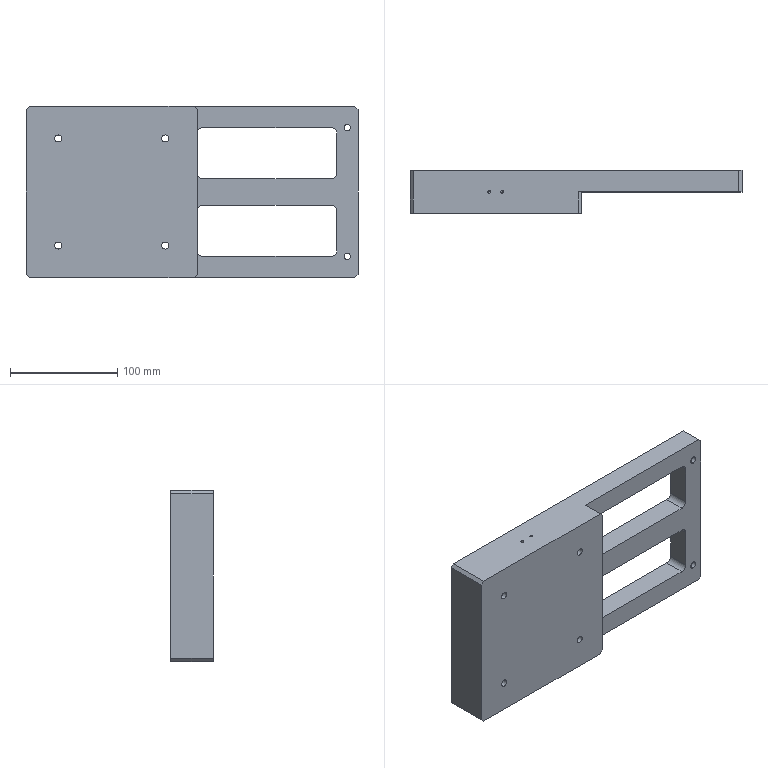Part | 1 solid | 56 faces | box 310 x 40 x 160 mm | volume 1242142 mm3 | plane 24 | cylinder 24 | cone 8 | commonest cylinder face diameters 10 x8 6.6 x4 6.8 x4 11 x4 2.5 x2 6 x2
STEP:
#1=CARTESIAN_POINT('',(125.,20.,60.));
#2=VERTEX_POINT('',#1);
#3=CARTESIAN_POINT('',(5.,20.,60.));
#4=VERTEX_POINT('',#3);
#5=CARTESIAN_POINT('',(5.,20.,60.));
#6=DIRECTION('',(-1.,0.,0.));
#7=VECTOR('',#6,1000.);
#8=LINE('',#5,#7);
#9=EDGE_CURVE('',#2,#4,#8,.T.);
#10=ORIENTED_EDGE('',*,*,#9,.T.);
#11=CARTESIAN_POINT('',(5.,40.,60.));
#12=VERTEX_POINT('',#11);
#13=CARTESIAN_POINT('',(5.,40.,60.));
#14=DIRECTION('',(0.,-1.,0.));
#15=VECTOR('',#14,1000.);
#16=LINE('',#13,#15);
#17=EDGE_CURVE('',#12,#4,#16,.T.);
#18=ORIENTED_EDGE('',*,*,#17,.F.);
#19=CARTESIAN_POINT('',(125.,40.,60.));
#20=VERTEX_POINT('',#19);
#21=CARTESIAN_POINT('',(5.,40.,60.));
#22=DIRECTION('',(-1.,0.,0.));
#23=VECTOR('',#22,1000.);
#24=LINE('',#21,#23);
#25=EDGE_CURVE('',#20,#12,#24,.T.);
#26=ORIENTED_EDGE('',*,*,#25,.F.);
#27=CARTESIAN_POINT('',(125.,40.,60.));
#28=DIRECTION('',(0.,-1.,0.));
#29=VECTOR('',#28,1000.);
#30=LINE('',#27,#29);
#31=EDGE_CURVE('',#20,#2,#30,.T.);
#32=ORIENTED_EDGE('',*,*,#31,.T.);
#33=EDGE_LOOP('',(#10,#18,#26,#32));
#34=FACE_BOUND('',#33,.T.);
#35=CARTESIAN_POINT('',(5.,40.,60.));
#36=DIRECTION('',(0.,0.,1.));
#37=DIRECTION('',(1.,0.,0.));
#38=AXIS2_PLACEMENT_3D('',#35,#36,#37);
#39=PLANE('',#38);
#40=ADVANCED_FACE('',(#34),#39,.F.);
#41=CARTESIAN_POINT('',(0.,20.,55.));
#42=VERTEX_POINT('',#41);
#43=CARTESIAN_POINT('',(5.,20.,55.));
#44=DIRECTION('',(0.,-1.,0.));
#45=DIRECTION('',(0.,0.,1.));
#46=AXIS2_PLACEMENT_3D('',#43,#44,#45);
#47=CIRCLE('',#46,5.);
#48=EDGE_CURVE('',#4,#42,#47,.T.);
#49=ORIENTED_EDGE('',*,*,#48,.T.);
#50=CARTESIAN_POINT('',(0.,40.,55.));
#51=VERTEX_POINT('',#50);
#52=CARTESIAN_POINT('',(0.,40.,55.));
#53=DIRECTION('',(0.,-1.,0.));
#54=VECTOR('',#53,1000.);
#55=LINE('',#52,#54);
#56=EDGE_CURVE('',#51,#42,#55,.T.);
#57=ORIENTED_EDGE('',*,*,#56,.F.);
#58=CARTESIAN_POINT('',(5.,40.,55.));
#59=DIRECTION('',(0.,-1.,0.));
#60=DIRECTION('',(0.,0.,1.));
#61=AXIS2_PLACEMENT_3D('',#58,#59,#60);
#62=CIRCLE('',#61,5.);
#63=EDGE_CURVE('',#12,#51,#62,.T.);
#64=ORIENTED_EDGE('',*,*,#63,.F.);
#65=ORIENTED_EDGE('',*,*,#17,.T.);
#66=EDGE_LOOP('',(#49,#57,#64,#65));
#67=FACE_BOUND('',#66,.T.);
#68=CARTESIAN_POINT('',(5.,40.,55.));
#69=DIRECTION('',(0.,-1.,0.));
#70=DIRECTION('',(0.,0.,-1.));
#71=AXIS2_PLACEMENT_3D('',#68,#69,#70);
#72=CYLINDRICAL_SURFACE('',#71,5.);
#73=ADVANCED_FACE('',(#67),#72,.F.);
#74=CARTESIAN_POINT('',(0.,20.,17.5));
#75=VERTEX_POINT('',#74);
#76=CARTESIAN_POINT('',(5.,20.,12.5));
#77=VERTEX_POINT('',#76);
#78=CARTESIAN_POINT('',(5.,20.,17.5));
#79=DIRECTION('',(0.,-1.,0.));
#80=DIRECTION('',(0.,0.,1.));
#81=AXIS2_PLACEMENT_3D('',#78,#79,#80);
#82=CIRCLE('',#81,5.);
#83=EDGE_CURVE('',#75,#77,#82,.T.);
#84=ORIENTED_EDGE('',*,*,#83,.T.);
#85=CARTESIAN_POINT('',(5.,40.,12.5));
#86=VERTEX_POINT('',#85);
#87=CARTESIAN_POINT('',(5.,40.,12.5));
#88=DIRECTION('',(0.,-1.,0.));
#89=VECTOR('',#88,1000.);
#90=LINE('',#87,#89);
#91=EDGE_CURVE('',#86,#77,#90,.T.);
#92=ORIENTED_EDGE('',*,*,#91,.F.);
#93=CARTESIAN_POINT('',(0.,40.,17.5));
#94=VERTEX_POINT('',#93);
#95=CARTESIAN_POINT('',(5.,40.,17.5));
#96=DIRECTION('',(0.,-1.,0.));
#97=DIRECTION('',(0.,0.,1.));
#98=AXIS2_PLACEMENT_3D('',#95,#96,#97);
#99=CIRCLE('',#98,5.);
#100=EDGE_CURVE('',#94,#86,#99,.T.);
#101=ORIENTED_EDGE('',*,*,#100,.F.);
#102=CARTESIAN_POINT('',(0.,40.,17.5));
#103=DIRECTION('',(0.,-1.,0.));
#104=VECTOR('',#103,1000.);
#105=LINE('',#102,#104);
#106=EDGE_CURVE('',#94,#75,#105,.T.);
#107=ORIENTED_EDGE('',*,*,#106,.T.);
#108=EDGE_LOOP('',(#84,#92,#101,#107));
#109=FACE_BOUND('',#108,.T.);
#110=CARTESIAN_POINT('',(5.,40.,17.5));
#111=DIRECTION('',(0.,-1.,0.));
#112=DIRECTION('',(0.,0.,-1.));
#113=AXIS2_PLACEMENT_3D('',#110,#111,#112);
#114=CYLINDRICAL_SURFACE('',#113,5.);
#115=ADVANCED_FACE('',(#109),#114,.F.);
#116=CARTESIAN_POINT('',(125.,20.,12.5));
#117=VERTEX_POINT('',#116);
#118=CARTESIAN_POINT('',(5.,20.,12.5));
#119=DIRECTION('',(1.,0.,0.));
#120=VECTOR('',#119,1000.);
#121=LINE('',#118,#120);
#122=EDGE_CURVE('',#77,#117,#121,.T.);
#123=ORIENTED_EDGE('',*,*,#122,.T.);
#124=CARTESIAN_POINT('',(125.,40.,12.5));
#125=VERTEX_POINT('',#124);
#126=CARTESIAN_POINT('',(125.,40.,12.5));
#127=DIRECTION('',(0.,-1.,0.));
#128=VECTOR('',#127,1000.);
#129=LINE('',#126,#128);
#130=EDGE_CURVE('',#125,#117,#129,.T.);
#131=ORIENTED_EDGE('',*,*,#130,.F.);
#132=CARTESIAN_POINT('',(5.,40.,12.5));
#133=DIRECTION('',(1.,0.,0.));
#134=VECTOR('',#133,1000.);
#135=LINE('',#132,#134);
#136=EDGE_CURVE('',#86,#125,#135,.T.);
#137=ORIENTED_EDGE('',*,*,#136,.F.);
#138=ORIENTED_EDGE('',*,*,#91,.T.);
#139=EDGE_LOOP('',(#123,#131,#137,#138));
#140=FACE_BOUND('',#139,.T.);
#141=CARTESIAN_POINT('',(5.,40.,12.5));
#142=DIRECTION('',(0.,0.,-1.));
#143=DIRECTION('',(-1.,0.,0.));
#144=AXIS2_PLACEMENT_3D('',#141,#142,#143);
#145=PLANE('',#144);
#146=ADVANCED_FACE('',(#140),#145,.F.);
#147=CARTESIAN_POINT('',(130.,20.,17.5));
#148=VERTEX_POINT('',#147);
#149=CARTESIAN_POINT('',(125.,20.,17.5));
#150=DIRECTION('',(0.,-1.,0.));
#151=DIRECTION('',(0.,0.,-1.));
#152=AXIS2_PLACEMENT_3D('',#149,#150,#151);
#153=CIRCLE('',#152,5.);
#154=EDGE_CURVE('',#117,#148,#153,.T.);
#155=ORIENTED_EDGE('',*,*,#154,.T.);
#156=CARTESIAN_POINT('',(130.,40.,17.5));
#157=VERTEX_POINT('',#156);
#158=CARTESIAN_POINT('',(130.,40.,17.5));
#159=DIRECTION('',(0.,-1.,0.));
#160=VECTOR('',#159,1000.);
#161=LINE('',#158,#160);
#162=EDGE_CURVE('',#157,#148,#161,.T.);
#163=ORIENTED_EDGE('',*,*,#162,.F.);
#164=CARTESIAN_POINT('',(125.,40.,17.5));
#165=DIRECTION('',(0.,-1.,0.));
#166=DIRECTION('',(0.,0.,-1.));
#167=AXIS2_PLACEMENT_3D('',#164,#165,#166);
#168=CIRCLE('',#167,5.);
#169=EDGE_CURVE('',#125,#157,#168,.T.);
#170=ORIENTED_EDGE('',*,*,#169,.F.);
#171=ORIENTED_EDGE('',*,*,#130,.T.);
#172=EDGE_LOOP('',(#155,#163,#170,#171));
#173=FACE_BOUND('',#172,.T.);
#174=CARTESIAN_POINT('',(125.,40.,17.5));
#175=DIRECTION('',(0.,-1.,0.));
#176=DIRECTION('',(0.,0.,-1.));
#177=AXIS2_PLACEMENT_3D('',#174,#175,#176);
#178=CYLINDRICAL_SURFACE('',#177,5.);
#179=ADVANCED_FACE('',(#173),#178,.F.);
#180=CARTESIAN_POINT('',(130.,20.,55.));
#181=VERTEX_POINT('',#180);
#182=CARTESIAN_POINT('',(130.,20.,17.5));
#183=DIRECTION('',(0.,0.,1.));
#184=VECTOR('',#183,1000.);
#185=LINE('',#182,#184);
#186=EDGE_CURVE('',#148,#181,#185,.T.);
#187=ORIENTED_EDGE('',*,*,#186,.T.);
#188=CARTESIAN_POINT('',(130.,40.,55.));
#189=VERTEX_POINT('',#188);
#190=CARTESIAN_POINT('',(130.,40.,55.));
#191=DIRECTION('',(0.,-1.,0.));
#192=VECTOR('',#191,1000.);
#193=LINE('',#190,#192);
#194=EDGE_CURVE('',#189,#181,#193,.T.);
#195=ORIENTED_EDGE('',*,*,#194,.F.);
#196=CARTESIAN_POINT('',(130.,40.,17.5));
#197=DIRECTION('',(0.,0.,1.));
#198=VECTOR('',#197,1000.);
#199=LINE('',#196,#198);
#200=EDGE_CURVE('',#157,#189,#199,.T.);
#201=ORIENTED_EDGE('',*,*,#200,.F.);
#202=ORIENTED_EDGE('',*,*,#162,.T.);
#203=EDGE_LOOP('',(#187,#195,#201,#202));
#204=FACE_BOUND('',#203,.T.);
#205=CARTESIAN_POINT('',(130.,40.,17.5));
#206=DIRECTION('',(1.,0.,0.));
#207=DIRECTION('',(0.,0.,-1.));
#208=AXIS2_PLACEMENT_3D('',#205,#206,#207);
#209=PLANE('',#208);
#210=ADVANCED_FACE('',(#204),#209,.F.);
#211=CARTESIAN_POINT('',(125.,20.,55.));
#212=DIRECTION('',(0.,-1.,0.));
#213=DIRECTION('',(0.,0.,1.));
#214=AXIS2_PLACEMENT_3D('',#211,#212,#213);
#215=CIRCLE('',#214,5.);
#216=EDGE_CURVE('',#181,#2,#215,.T.);
#217=ORIENTED_EDGE('',*,*,#216,.T.);
#218=ORIENTED_EDGE('',*,*,#31,.F.);
#219=CARTESIAN_POINT('',(125.,40.,55.));
#220=DIRECTION('',(0.,-1.,0.));
#221=DIRECTION('',(0.,0.,1.));
#222=AXIS2_PLACEMENT_3D('',#219,#220,#221);
#223=CIRCLE('',#222,5.);
#224=EDGE_CURVE('',#189,#20,#223,.T.);
#225=ORIENTED_EDGE('',*,*,#224,.F.);
#226=ORIENTED_EDGE('',*,*,#194,.T.);
#227=EDGE_LOOP('',(#217,#218,#225,#226));
#228=FACE_BOUND('',#227,.T.);
#229=CARTESIAN_POINT('',(125.,40.,55.));
#230=DIRECTION('',(0.,-1.,0.));
#231=DIRECTION('',(0.,0.,-1.));
#232=AXIS2_PLACEMENT_3D('',#229,#230,#231);
#233=CYLINDRICAL_SURFACE('',#232,5.);
#234=ADVANCED_FACE('',(#228),#233,.F.);
#235=CARTESIAN_POINT('',(5.,20.,-60.));
#236=VERTEX_POINT('',#235);
#237=CARTESIAN_POINT('',(125.,20.,-60.));
#238=VERTEX_POINT('',#237);
#239=CARTESIAN_POINT('',(5.,20.,-60.));
#240=DIRECTION('',(1.,0.,0.));
#241=VECTOR('',#240,1000.);
#242=LINE('',#239,#241);
#243=EDGE_CURVE('',#236,#238,#242,.T.);
#244=ORIENTED_EDGE('',*,*,#243,.T.);
#245=CARTESIAN_POINT('',(125.,40.,-60.));
#246=VERTEX_POINT('',#245);
#247=CARTESIAN_POINT('',(125.,40.,-60.));
#248=DIRECTION('',(0.,-1.,0.));
#249=VECTOR('',#248,1000.);
#250=LINE('',#247,#249);
#251=EDGE_CURVE('',#246,#238,#250,.T.);
#252=ORIENTED_EDGE('',*,*,#251,.F.);
#253=CARTESIAN_POINT('',(5.,40.,-60.));
#254=VERTEX_POINT('',#253);
#255=CARTESIAN_POINT('',(5.,40.,-60.));
#256=DIRECTION('',(1.,0.,0.));
#257=VECTOR('',#256,1000.);
#258=LINE('',#255,#257);
#259=EDGE_CURVE('',#254,#246,#258,.T.);
#260=ORIENTED_EDGE('',*,*,#259,.F.);
#261=CARTESIAN_POINT('',(5.,40.,-60.));
#262=DIRECTION('',(0.,-1.,0.));
#263=VECTOR('',#262,1000.);
#264=LINE('',#261,#263);
#265=EDGE_CURVE('',#254,#236,#264,.T.);
#266=ORIENTED_EDGE('',*,*,#265,.T.);
#267=EDGE_LOOP('',(#244,#252,#260,#266));
#268=FACE_BOUND('',#267,.T.);
#269=CARTESIAN_POINT('',(5.,40.,-60.));
#270=DIRECTION('',(0.,0.,-1.));
#271=DIRECTION('',(-1.,0.,0.));
#272=AXIS2_PLACEMENT_3D('',#269,#270,#271);
#273=PLANE('',#272);
#274=ADVANCED_FACE('',(#268),#273,.F.);
#275=CARTESIAN_POINT('',(130.,20.,-55.));
#276=VERTEX_POINT('',#275);
#277=CARTESIAN_POINT('',(125.,20.,-55.));
#278=DIRECTION('',(0.,-1.,0.));
#279=DIRECTION('',(0.,0.,-1.));
#280=AXIS2_PLACEMENT_3D('',#277,#278,#279);
#281=CIRCLE('',#280,5.);
#282=EDGE_CURVE('',#238,#276,#281,.T.);
#283=ORIENTED_EDGE('',*,*,#282,.T.);
#284=CARTESIAN_POINT('',(130.,40.,-55.));
#285=VERTEX_POINT('',#284);
#286=CARTESIAN_POINT('',(130.,40.,-55.));
#287=DIRECTION('',(0.,-1.,0.));
#288=VECTOR('',#287,1000.);
#289=LINE('',#286,#288);
#290=EDGE_CURVE('',#285,#276,#289,.T.);
#291=ORIENTED_EDGE('',*,*,#290,.F.);
#292=CARTESIAN_POINT('',(125.,40.,-55.));
#293=DIRECTION('',(0.,-1.,0.));
#294=DIRECTION('',(0.,0.,-1.));
#295=AXIS2_PLACEMENT_3D('',#292,#293,#294);
#296=CIRCLE('',#295,5.);
#297=EDGE_CURVE('',#246,#285,#296,.T.);
#298=ORIENTED_EDGE('',*,*,#297,.F.);
#299=ORIENTED_EDGE('',*,*,#251,.T.);
#300=EDGE_LOOP('',(#283,#291,#298,#299));
#301=FACE_BOUND('',#300,.T.);
#302=CARTESIAN_POINT('',(125.,40.,-55.));
#303=DIRECTION('',(0.,-1.,0.));
#304=DIRECTION('',(0.,0.,-1.));
#305=AXIS2_PLACEMENT_3D('',#302,#303,#304);
#306=CYLINDRICAL_SURFACE('',#305,5.);
#307=ADVANCED_FACE('',(#301),#306,.F.);
#308=CARTESIAN_POINT('',(130.,20.,-17.5));
#309=VERTEX_POINT('',#308);
#310=CARTESIAN_POINT('',(130.,20.,17.5));
#311=DIRECTION('',(0.,0.,1.));
#312=VECTOR('',#311,1000.);
#313=LINE('',#310,#312);
#314=EDGE_CURVE('',#276,#309,#313,.T.);
#315=ORIENTED_EDGE('',*,*,#314,.T.);
#316=CARTESIAN_POINT('',(130.,40.,-17.5));
#317=VERTEX_POINT('',#316);
#318=CARTESIAN_POINT('',(130.,40.,-17.5));
#319=DIRECTION('',(0.,-1.,0.));
#320=VECTOR('',#319,1000.);
#321=LINE('',#318,#320);
#322=EDGE_CURVE('',#317,#309,#321,.T.);
#323=ORIENTED_EDGE('',*,*,#322,.F.);
#324=CARTESIAN_POINT('',(130.,40.,80.));
#325=DIRECTION('',(0.,0.,1.));
#326=VECTOR('',#325,1000.);
#327=LINE('',#324,#326);
#328=EDGE_CURVE('',#285,#317,#327,.T.);
#329=ORIENTED_EDGE('',*,*,#328,.F.);
#330=ORIENTED_EDGE('',*,*,#290,.T.);
#331=EDGE_LOOP('',(#315,#323,#329,#330));
#332=FACE_BOUND('',#331,.T.);
#333=CARTESIAN_POINT('',(130.,40.,17.5));
#334=DIRECTION('',(1.,0.,0.));
#335=DIRECTION('',(0.,0.,-1.));
#336=AXIS2_PLACEMENT_3D('',#333,#334,#335);
#337=PLANE('',#336);
#338=ADVANCED_FACE('',(#332),#337,.F.);
#339=CARTESIAN_POINT('',(125.,20.,-12.5));
#340=VERTEX_POINT('',#339);
#341=CARTESIAN_POINT('',(125.,20.,-17.5));
#342=DIRECTION('',(0.,-1.,0.));
#343=DIRECTION('',(0.,0.,1.));
#344=AXIS2_PLACEMENT_3D('',#341,#342,#343);
#345=CIRCLE('',#344,5.);
#346=EDGE_CURVE('',#309,#340,#345,.T.);
#347=ORIENTED_EDGE('',*,*,#346,.T.);
#348=CARTESIAN_POINT('',(125.,40.,-12.5));
#349=VERTEX_POINT('',#348);
#350=CARTESIAN_POINT('',(125.,40.,-12.5));
#351=DIRECTION('',(0.,-1.,0.));
#352=VECTOR('',#351,1000.);
#353=LINE('',#350,#352);
#354=EDGE_CURVE('',#349,#340,#353,.T.);
#355=ORIENTED_EDGE('',*,*,#354,.F.);
#356=CARTESIAN_POINT('',(125.,40.,-17.5));
#357=DIRECTION('',(0.,-1.,0.));
#358=DIRECTION('',(0.,0.,1.));
#359=AXIS2_PLACEMENT_3D('',#356,#357,#358);
#360=CIRCLE('',#359,5.);
#361=EDGE_CURVE('',#317,#349,#360,.T.);
#362=ORIENTED_EDGE('',*,*,#361,.F.);
#363=ORIENTED_EDGE('',*,*,#322,.T.);
#364=EDGE_LOOP('',(#347,#355,#362,#363));
#365=FACE_BOUND('',#364,.T.);
#366=CARTESIAN_POINT('',(125.,40.,-17.5));
#367=DIRECTION('',(0.,-1.,0.));
#368=DIRECTION('',(0.,0.,-1.));
#369=AXIS2_PLACEMENT_3D('',#366,#367,#368);
#370=CYLINDRICAL_SURFACE('',#369,5.);
#371=ADVANCED_FACE('',(#365),#370,.F.);
#372=CARTESIAN_POINT('',(5.,20.,-12.5));
#373=VERTEX_POINT('',#372);
#374=CARTESIAN_POINT('',(5.,20.,-12.5));
#375=DIRECTION('',(-1.,0.,0.));
#376=VECTOR('',#375,1000.);
#377=LINE('',#374,#376);
#378=EDGE_CURVE('',#340,#373,#377,.T.);
#379=ORIENTED_EDGE('',*,*,#378,.T.);
#380=CARTESIAN_POINT('',(5.,40.,-12.5));
#381=VERTEX_POINT('',#380);
#382=CARTESIAN_POINT('',(5.,40.,-12.5));
#383=DIRECTION('',(0.,-1.,0.));
#384=VECTOR('',#383,1000.);
#385=LINE('',#382,#384);
#386=EDGE_CURVE('',#381,#373,#385,.T.);
#387=ORIENTED_EDGE('',*,*,#386,.F.);
#388=CARTESIAN_POINT('',(5.,40.,-12.5));
#389=DIRECTION('',(-1.,0.,0.));
#390=VECTOR('',#389,1000.);
#391=LINE('',#388,#390);
#392=EDGE_CURVE('',#349,#381,#391,.T.);
#393=ORIENTED_EDGE('',*,*,#392,.F.);
#394=ORIENTED_EDGE('',*,*,#354,.T.);
#395=EDGE_LOOP('',(#379,#387,#393,#394));
#396=FACE_BOUND('',#395,.T.);
#397=CARTESIAN_POINT('',(5.,40.,-12.5));
#398=DIRECTION('',(0.,0.,1.));
#399=DIRECTION('',(1.,0.,0.));
#400=AXIS2_PLACEMENT_3D('',#397,#398,#399);
#401=PLANE('',#400);
#402=ADVANCED_FACE('',(#396),#401,.F.);
#403=CARTESIAN_POINT('',(0.,20.,-17.5));
#404=VERTEX_POINT('',#403);
#405=CARTESIAN_POINT('',(5.,20.,-17.5));
#406=DIRECTION('',(0.,-1.,0.));
#407=DIRECTION('',(0.,0.,-1.));
#408=AXIS2_PLACEMENT_3D('',#405,#406,#407);
#409=CIRCLE('',#408,5.);
#410=EDGE_CURVE('',#373,#404,#409,.T.);
#411=ORIENTED_EDGE('',*,*,#410,.T.);
#412=CARTESIAN_POINT('',(0.,40.,-17.5));
#413=VERTEX_POINT('',#412);
#414=CARTESIAN_POINT('',(0.,40.,-17.5));
#415=DIRECTION('',(0.,-1.,0.));
#416=VECTOR('',#415,1000.);
#417=LINE('',#414,#416);
#418=EDGE_CURVE('',#413,#404,#417,.T.);
#419=ORIENTED_EDGE('',*,*,#418,.F.);
#420=CARTESIAN_POINT('',(5.,40.,-17.5));
#421=DIRECTION('',(0.,-1.,0.));
#422=DIRECTION('',(0.,0.,-1.));
#423=AXIS2_PLACEMENT_3D('',#420,#421,#422);
#424=CIRCLE('',#423,5.);
#425=EDGE_CURVE('',#381,#413,#424,.T.);
#426=ORIENTED_EDGE('',*,*,#425,.F.);
#427=ORIENTED_EDGE('',*,*,#386,.T.);
#428=EDGE_LOOP('',(#411,#419,#426,#427));
#429=FACE_BOUND('',#428,.T.);
#430=CARTESIAN_POINT('',(5.,40.,-17.5));
#431=DIRECTION('',(0.,-1.,0.));
#432=DIRECTION('',(0.,0.,-1.));
#433=AXIS2_PLACEMENT_3D('',#430,#431,#432);
#434=CYLINDRICAL_SURFACE('',#433,5.);
#435=ADVANCED_FACE('',(#429),#434,.F.);
#436=CARTESIAN_POINT('',(0.,20.,-55.));
#437=VERTEX_POINT('',#436);
#438=CARTESIAN_POINT('',(5.,20.,-55.));
#439=DIRECTION('',(0.,-1.,0.));
#440=DIRECTION('',(0.,0.,-1.));
#441=AXIS2_PLACEMENT_3D('',#438,#439,#440);
#442=CIRCLE('',#441,5.);
#443=EDGE_CURVE('',#437,#236,#442,.T.);
#444=ORIENTED_EDGE('',*,*,#443,.T.);
#445=ORIENTED_EDGE('',*,*,#265,.F.);
#446=CARTESIAN_POINT('',(0.,40.,-55.));
#447=VERTEX_POINT('',#446);
#448=CARTESIAN_POINT('',(5.,40.,-55.));
#449=DIRECTION('',(0.,-1.,0.));
#450=DIRECTION('',(0.,0.,-1.));
#451=AXIS2_PLACEMENT_3D('',#448,#449,#450);
#452=CIRCLE('',#451,5.);
#453=EDGE_CURVE('',#447,#254,#452,.T.);
#454=ORIENTED_EDGE('',*,*,#453,.F.);
#455=CARTESIAN_POINT('',(0.,40.,-55.));
#456=DIRECTION('',(0.,-1.,0.));
#457=VECTOR('',#456,1000.);
#458=LINE('',#455,#457);
#459=EDGE_CURVE('',#447,#437,#458,.T.);
#460=ORIENTED_EDGE('',*,*,#459,.T.);
#461=EDGE_LOOP('',(#444,#445,#454,#460));
#462=FACE_BOUND('',#461,.T.);
#463=CARTESIAN_POINT('',(5.,40.,-55.));
#464=DIRECTION('',(0.,-1.,0.));
#465=DIRECTION('',(0.,0.,-1.));
#466=AXIS2_PLACEMENT_3D('',#463,#464,#465);
#467=CYLINDRICAL_SURFACE('',#466,5.);
#468=ADVANCED_FACE('',(#462),#467,.F.);
#469=CARTESIAN_POINT('',(-30.,15.,55.5));
#470=VERTEX_POINT('',#469);
#471=CARTESIAN_POINT('',(-30.,15.,50.));
#472=DIRECTION('',(0.,1.,0.));
#473=DIRECTION('',(0.,0.,1.));
#474=AXIS2_PLACEMENT_3D('',#471,#472,#473);
#475=CIRCLE('',#474,5.5);
#476=EDGE_CURVE('',#470,#470,#475,.T.);
#477=ORIENTED_EDGE('',*,*,#476,.T.);
#478=EDGE_LOOP('',(#477));
#479=FACE_BOUND('',#478,.T.);
#480=CARTESIAN_POINT('',(-30.,15.,53.3));
#481=VERTEX_POINT('',#480);
#482=CARTESIAN_POINT('',(-30.,15.,50.));
#483=DIRECTION('',(0.,1.,0.));
#484=DIRECTION('',(0.,0.,1.));
#485=AXIS2_PLACEMENT_3D('',#482,#483,#484);
#486=CIRCLE('',#485,3.3);
#487=EDGE_CURVE('',#481,#481,#486,.T.);
#488=ORIENTED_EDGE('',*,*,#487,.F.);
#489=EDGE_LOOP('',(#488));
#490=FACE_BOUND('',#489,.T.);
#491=CARTESIAN_POINT('',(-26.7,15.,50.));
#492=DIRECTION('',(0.,-1.,0.));
#493=DIRECTION('',(0.,0.,-1.));
#494=AXIS2_PLACEMENT_3D('',#491,#492,#493);
#495=PLANE('',#494);
#496=ADVANCED_FACE('',(#479,#490),#495,.F.);
#497=CARTESIAN_POINT('',(-130.,15.,44.5));
#498=VERTEX_POINT('',#497);
#499=CARTESIAN_POINT('',(-130.,15.,50.));
#500=DIRECTION('',(0.,1.,0.));
#501=DIRECTION('',(0.,0.,-1.));
#502=AXIS2_PLACEMENT_3D('',#499,#500,#501);
#503=CIRCLE('',#502,5.5);
#504=EDGE_CURVE('',#498,#498,#503,.T.);
#505=ORIENTED_EDGE('',*,*,#504,.T.);
#506=EDGE_LOOP('',(#505));
#507=FACE_BOUND('',#506,.T.);
#508=CARTESIAN_POINT('',(-130.,15.,46.7));
#509=VERTEX_POINT('',#508);
#510=CARTESIAN_POINT('',(-130.,15.,50.));
#511=DIRECTION('',(0.,1.,0.));
#512=DIRECTION('',(0.,0.,-1.));
#513=AXIS2_PLACEMENT_3D('',#510,#511,#512);
#514=CIRCLE('',#513,3.3);
#515=EDGE_CURVE('',#509,#509,#514,.T.);
#516=ORIENTED_EDGE('',*,*,#515,.F.);
#517=EDGE_LOOP('',(#516));
#518=FACE_BOUND('',#517,.T.);
#519=CARTESIAN_POINT('',(-26.7,15.,50.));
#520=DIRECTION('',(0.,-1.,0.));
#521=DIRECTION('',(0.,0.,-1.));
#522=AXIS2_PLACEMENT_3D('',#519,#520,#521);
#523=PLANE('',#522);
#524=ADVANCED_FACE('',(#507,#518),#523,.F.);
#525=CARTESIAN_POINT('',(-130.,15.,-55.5));
#526=VERTEX_POINT('',#525);
#527=CARTESIAN_POINT('',(-130.,15.,-50.));
#528=DIRECTION('',(0.,1.,0.));
#529=DIRECTION('',(0.,0.,-1.));
#530=AXIS2_PLACEMENT_3D('',#527,#528,#529);
#531=CIRCLE('',#530,5.5);
#532=EDGE_CURVE('',#526,#526,#531,.T.);
#533=ORIENTED_EDGE('',*,*,#532,.T.);
#534=EDGE_LOOP('',(#533));
#535=FACE_BOUND('',#534,.T.);
#536=CARTESIAN_POINT('',(-130.,15.,-53.3));
#537=VERTEX_POINT('',#536);
#538=CARTESIAN_POINT('',(-130.,15.,-50.));
#539=DIRECTION('',(0.,1.,0.));
#540=DIRECTION('',(0.,0.,-1.));
#541=AXIS2_PLACEMENT_3D('',#538,#539,#540);
#542=CIRCLE('',#541,3.3);
#543=EDGE_CURVE('',#537,#537,#542,.T.);
#544=ORIENTED_EDGE('',*,*,#543,.F.);
#545=EDGE_LOOP('',(#544));
#546=FACE_BOUND('',#545,.T.);
#547=CARTESIAN_POINT('',(-26.7,15.,50.));
#548=DIRECTION('',(0.,-1.,0.));
#549=DIRECTION('',(0.,0.,-1.));
#550=AXIS2_PLACEMENT_3D('',#547,#548,#549);
#551=PLANE('',#550);
#552=ADVANCED_FACE('',(#535,#546),#551,.F.);
#553=CARTESIAN_POINT('',(-30.,15.,-55.5));
#554=VERTEX_POINT('',#553);
#555=CARTESIAN_POINT('',(-30.,15.,-50.));
#556=DIRECTION('',(0.,1.,0.));
#557=DIRECTION('',(0.,0.,-1.));
#558=AXIS2_PLACEMENT_3D('',#555,#556,#557);
#559=CIRCLE('',#558,5.5);
#560=EDGE_CURVE('',#554,#554,#559,.T.);
#561=ORIENTED_EDGE('',*,*,#560,.T.);
#562=EDGE_LOOP('',(#561));
#563=FACE_BOUND('',#562,.T.);
#564=CARTESIAN_POINT('',(-30.,15.,-53.3));
#565=VERTEX_POINT('',#564);
#566=CARTESIAN_POINT('',(-30.,15.,-50.));
#567=DIRECTION('',(0.,1.,0.));
#568=DIRECTION('',(0.,0.,-1.));
#569=AXIS2_PLACEMENT_3D('',#566,#567,#568);
#570=CIRCLE('',#569,3.3);
#571=EDGE_CURVE('',#565,#565,#570,.T.);
#572=ORIENTED_EDGE('',*,*,#571,.F.);
#573=EDGE_LOOP('',(#572));
#574=FACE_BOUND('',#573,.T.);
#575=CARTESIAN_POINT('',(-26.7,15.,50.));
#576=DIRECTION('',(0.,-1.,0.));
#577=DIRECTION('',(0.,0.,-1.));
#578=AXIS2_PLACEMENT_3D('',#575,#576,#577);
#579=PLANE('',#578);
#580=ADVANCED_FACE('',(#563,#574),#579,.F.);
#581=CARTESIAN_POINT('',(147.,20.,-80.));
#582=VERTEX_POINT('',#581);
#583=CARTESIAN_POINT('',(150.,20.,-77.));
#584=VERTEX_POINT('',#583);
#585=CARTESIAN_POINT('',(150.,20.,-77.));
#586=DIRECTION('',(0.7071,0.,0.7071));
#587=VECTOR('',#586,1000.);
#588=LINE('',#585,#587);
#589=EDGE_CURVE('',#582,#584,#588,.T.);
#590=ORIENTED_EDGE('',*,*,#589,.F.);
#591=CARTESIAN_POINT('',(147.,40.,-80.));
#592=VERTEX_POINT('',#591);
#593=CARTESIAN_POINT('',(147.,20.,-80.));
#594=DIRECTION('',(0.,-1.,0.));
#595=VECTOR('',#594,1000.);
#596=LINE('',#593,#595);
#597=EDGE_CURVE('',#592,#582,#596,.T.);
#598=ORIENTED_EDGE('',*,*,#597,.F.);
#599=CARTESIAN_POINT('',(150.,40.,-77.));
#600=VERTEX_POINT('',#599);
#601=CARTESIAN_POINT('',(150.,40.,-77.));
#602=DIRECTION('',(-0.7071,0.,-0.7071));
#603=VECTOR('',#602,1000.);
#604=LINE('',#601,#603);
#605=EDGE_CURVE('',#600,#592,#604,.T.);
#606=ORIENTED_EDGE('',*,*,#605,.F.);
#607=CARTESIAN_POINT('',(150.,40.,-77.));
#608=DIRECTION('',(0.,1.,0.));
#609=VECTOR('',#608,1000.);
#610=LINE('',#607,#609);
#611=EDGE_CURVE('',#584,#600,#610,.T.);
#612=ORIENTED_EDGE('',*,*,#611,.F.);
#613=EDGE_LOOP('',(#590,#598,#606,#612));
#614=FACE_BOUND('',#613,.T.);
#615=CARTESIAN_POINT('',(150.,20.,-77.));
#616=DIRECTION('',(0.7071,0.,-0.7071));
#617=DIRECTION('',(0.,-1.,0.));
#618=AXIS2_PLACEMENT_3D('',#615,#616,#617);
#619=PLANE('',#618);
#620=ADVANCED_FACE('',(#614),#619,.T.);
#621=CARTESIAN_POINT('',(150.,20.,77.));
#622=VERTEX_POINT('',#621);
#623=CARTESIAN_POINT('',(147.,20.,80.));
#624=VERTEX_POINT('',#623);
#625=CARTESIAN_POINT('',(147.,20.,80.));
#626=DIRECTION('',(-0.7071,0.,0.7071));
#627=VECTOR('',#626,1000.);
#628=LINE('',#625,#627);
#629=EDGE_CURVE('',#622,#624,#628,.T.);
#630=ORIENTED_EDGE('',*,*,#629,.F.);
#631=CARTESIAN_POINT('',(150.,40.,77.));
#632=VERTEX_POINT('',#631);
#633=CARTESIAN_POINT('',(150.,20.,77.));
#634=DIRECTION('',(0.,-1.,0.));
#635=VECTOR('',#634,1000.);
#636=LINE('',#633,#635);
#637=EDGE_CURVE('',#632,#622,#636,.T.);
#638=ORIENTED_EDGE('',*,*,#637,.F.);
#639=CARTESIAN_POINT('',(147.,40.,80.));
#640=VERTEX_POINT('',#639);
#641=CARTESIAN_POINT('',(147.,40.,80.));
#642=DIRECTION('',(0.7071,0.,-0.7071));
#643=VECTOR('',#642,1000.);
#644=LINE('',#641,#643);
#645=EDGE_CURVE('',#640,#632,#644,.T.);
#646=ORIENTED_EDGE('',*,*,#645,.F.);
#647=CARTESIAN_POINT('',(147.,0.,80.));
#648=DIRECTION('',(0.,1.,0.));
#649=VECTOR('',#648,1000.);
#650=LINE('',#647,#649);
#651=EDGE_CURVE('',#624,#640,#650,.T.);
#652=ORIENTED_EDGE('',*,*,#651,.F.);
#653=EDGE_LOOP('',(#630,#638,#646,#652));
#654=FACE_BOUND('',#653,.T.);
#655=CARTESIAN_POINT('',(147.,0.,80.));
#656=DIRECTION('',(-0.7071,0.,-0.7071));
#657=DIRECTION('',(0.,1.,0.));
#658=AXIS2_PLACEMENT_3D('',#655,#656,#657);
#659=PLANE('',#658);
#660=ADVANCED_FACE('',(#654),#659,.F.);
#661=CARTESIAN_POINT('',(-157.,40.,-80.));
#662=VERTEX_POINT('',#661);
#663=CARTESIAN_POINT('',(-160.,40.,-77.));
#664=VERTEX_POINT('',#663);
#665=CARTESIAN_POINT('',(-160.,40.,-77.));
#666=DIRECTION('',(-0.7071,0.,0.7071));
#667=VECTOR('',#666,1000.);
#668=LINE('',#665,#667);
#669=EDGE_CURVE('',#662,#664,#668,.T.);
#670=ORIENTED_EDGE('',*,*,#669,.F.);
#671=CARTESIAN_POINT('',(-157.,0.,-80.));
#672=VERTEX_POINT('',#671);
#673=CARTESIAN_POINT('',(-157.,40.,-80.));
#674=DIRECTION('',(0.,1.,0.));
#675=VECTOR('',#674,1000.);
#676=LINE('',#673,#675);
#677=EDGE_CURVE('',#672,#662,#676,.T.);
#678=ORIENTED_EDGE('',*,*,#677,.F.);
#679=CARTESIAN_POINT('',(-160.,0.,-77.));
#680=VERTEX_POINT('',#679);
#681=CARTESIAN_POINT('',(-160.,0.,-77.));
#682=DIRECTION('',(0.7071,0.,-0.7071));
#683=VECTOR('',#682,1000.);
#684=LINE('',#681,#683);
#685=EDGE_CURVE('',#680,#672,#684,.T.);
#686=ORIENTED_EDGE('',*,*,#685,.F.);
#687=CARTESIAN_POINT('',(-160.,0.,-77.));
#688=DIRECTION('',(0.,-1.,0.));
#689=VECTOR('',#688,1000.);
#690=LINE('',#687,#689);
#691=EDGE_CURVE('',#664,#680,#690,.T.);
#692=ORIENTED_EDGE('',*,*,#691,.F.);
#693=EDGE_LOOP('',(#670,#678,#686,#692));
#694=FACE_BOUND('',#693,.T.);
#695=CARTESIAN_POINT('',(-160.,40.,-77.));
#696=DIRECTION('',(-0.7071,0.,-0.7071));
#697=DIRECTION('',(0.,1.,0.));
#698=AXIS2_PLACEMENT_3D('',#695,#696,#697);
#699=PLANE('',#698);
#700=ADVANCED_FACE('',(#694),#699,.T.);
#701=CARTESIAN_POINT('',(-160.,40.,77.));
#702=VERTEX_POINT('',#701);
#703=CARTESIAN_POINT('',(-157.,40.,80.));
#704=VERTEX_POINT('',#703);
#705=CARTESIAN_POINT('',(-157.,40.,80.));
#706=DIRECTION('',(0.7071,0.,0.7071));
#707=VECTOR('',#706,1000.);
#708=LINE('',#705,#707);
#709=EDGE_CURVE('',#702,#704,#708,.T.);
#710=ORIENTED_EDGE('',*,*,#709,.F.);
#711=CARTESIAN_POINT('',(-160.,0.,77.));
#712=VERTEX_POINT('',#711);
#713=CARTESIAN_POINT('',(-160.,40.,77.));
#714=DIRECTION('',(0.,1.,0.));
#715=VECTOR('',#714,1000.);
#716=LINE('',#713,#715);
#717=EDGE_CURVE('',#712,#702,#716,.T.);
#718=ORIENTED_EDGE('',*,*,#717,.F.);
#719=CARTESIAN_POINT('',(-157.,0.,80.));
#720=VERTEX_POINT('',#719);
#721=CARTESIAN_POINT('',(-157.,0.,80.));
#722=DIRECTION('',(-0.7071,0.,-0.7071));
#723=VECTOR('',#722,1000.);
#724=LINE('',#721,#723);
#725=EDGE_CURVE('',#720,#712,#724,.T.);
#726=ORIENTED_EDGE('',*,*,#725,.F.);
#727=CARTESIAN_POINT('',(-157.,0.,80.));
#728=DIRECTION('',(0.,-1.,0.));
#729=VECTOR('',#728,1000.);
#730=LINE('',#727,#729);
#731=EDGE_CURVE('',#704,#720,#730,.T.);
#732=ORIENTED_EDGE('',*,*,#731,.F.);
#733=EDGE_LOOP('',(#710,#718,#726,#732));
#734=FACE_BOUND('',#733,.T.);
#735=CARTESIAN_POINT('',(-157.,0.,80.));
#736=DIRECTION('',(0.7071,0.,-0.7071));
#737=DIRECTION('',(0.,-1.,0.));
#738=AXIS2_PLACEMENT_3D('',#735,#736,#737);
#739=PLANE('',#738);
#740=ADVANCED_FACE('',(#734),#739,.F.);
#741=CARTESIAN_POINT('',(-3.,0.,-80.));
#742=VERTEX_POINT('',#741);
#743=CARTESIAN_POINT('',(0.,0.,-77.));
#744=VERTEX_POINT('',#743);
#745=CARTESIAN_POINT('',(0.,0.,-77.));
#746=DIRECTION('',(0.7071,0.,0.7071));
#747=VECTOR('',#746,1000.);
#748=LINE('',#745,#747);
#749=EDGE_CURVE('',#742,#744,#748,.T.);
#750=ORIENTED_EDGE('',*,*,#749,.F.);
#751=CARTESIAN_POINT('',(-3.,20.,-80.));
#752=VERTEX_POINT('',#751);
#753=CARTESIAN_POINT('',(-3.,0.,-80.));
#754=DIRECTION('',(0.,-1.,0.));
#755=VECTOR('',#754,1000.);
#756=LINE('',#753,#755);
#757=EDGE_CURVE('',#752,#742,#756,.T.);
#758=ORIENTED_EDGE('',*,*,#757,.F.);
#759=CARTESIAN_POINT('',(0.,20.,-77.));
#760=VERTEX_POINT('',#759);
#761=CARTESIAN_POINT('',(78.5,20.,1.5));
#762=DIRECTION('',(-0.7071,0.,-0.7071));
#763=VECTOR('',#762,1000.);
#764=LINE('',#761,#763);
#765=EDGE_CURVE('',#760,#752,#764,.T.);
#766=ORIENTED_EDGE('',*,*,#765,.F.);
#767=CARTESIAN_POINT('',(0.,20.,-77.));
#768=DIRECTION('',(0.,1.,0.));
#769=VECTOR('',#768,1000.);
#770=LINE('',#767,#769);
#771=EDGE_CURVE('',#744,#760,#770,.T.);
#772=ORIENTED_EDGE('',*,*,#771,.F.);
#773=EDGE_LOOP('',(#750,#758,#766,#772));
#774=FACE_BOUND('',#773,.T.);
#775=CARTESIAN_POINT('',(0.,0.,-77.));
#776=DIRECTION('',(0.7071,0.,-0.7071));
#777=DIRECTION('',(0.,-1.,0.));
#778=AXIS2_PLACEMENT_3D('',#775,#776,#777);
#779=PLANE('',#778);
#780=ADVANCED_FACE('',(#774),#779,.T.);
#781=CARTESIAN_POINT('',(0.,0.,77.));
#782=VERTEX_POINT('',#781);
#783=CARTESIAN_POINT('',(-3.,0.,80.));
#784=VERTEX_POINT('',#783);
#785=CARTESIAN_POINT('',(-3.,0.,80.));
#786=DIRECTION('',(-0.7071,0.,0.7071));
#787=VECTOR('',#786,1000.);
#788=LINE('',#785,#787);
#789=EDGE_CURVE('',#782,#784,#788,.T.);
#790=ORIENTED_EDGE('',*,*,#789,.F.);
#791=CARTESIAN_POINT('',(0.,20.,77.));
#792=VERTEX_POINT('',#791);
#793=CARTESIAN_POINT('',(0.,0.,77.));
#794=DIRECTION('',(0.,-1.,0.));
#795=VECTOR('',#794,1000.);
#796=LINE('',#793,#795);
#797=EDGE_CURVE('',#792,#782,#796,.T.);
#798=ORIENTED_EDGE('',*,*,#797,.F.);
#799=CARTESIAN_POINT('',(-3.,20.,80.));
#800=VERTEX_POINT('',#799);
#801=CARTESIAN_POINT('',(-1.5,20.,78.5));
#802=DIRECTION('',(0.7071,0.,-0.7071));
#803=VECTOR('',#802,1000.);
#804=LINE('',#801,#803);
#805=EDGE_CURVE('',#800,#792,#804,.T.);
#806=ORIENTED_EDGE('',*,*,#805,.F.);
#807=CARTESIAN_POINT('',(-3.,0.,80.));
#808=DIRECTION('',(0.,1.,0.));
#809=VECTOR('',#808,1000.);
#810=LINE('',#807,#809);
#811=EDGE_CURVE('',#784,#800,#810,.T.);
#812=ORIENTED_EDGE('',*,*,#811,.F.);
#813=EDGE_LOOP('',(#790,#798,#806,#812));
#814=FACE_BOUND('',#813,.T.);
#815=CARTESIAN_POINT('',(-3.,0.,80.));
#816=DIRECTION('',(-0.7071,0.,-0.7071));
#817=DIRECTION('',(0.,1.,0.));
#818=AXIS2_PLACEMENT_3D('',#815,#816,#817);
#819=PLANE('',#818);
#820=ADVANCED_FACE('',(#814),#819,.F.);
#821=CARTESIAN_POINT('',(0.,20.,-80.));
#822=DIRECTION('',(1.,0.,0.));
#823=VECTOR('',#822,1000.);
#824=LINE('',#821,#823);
#825=EDGE_CURVE('',#752,#582,#824,.T.);
#826=ORIENTED_EDGE('',*,*,#825,.F.);
#827=ORIENTED_EDGE('',*,*,#757,.T.);
#828=CARTESIAN_POINT('',(-160.,0.,-80.));
#829=DIRECTION('',(1.,0.,0.));
#830=VECTOR('',#829,1000.);
#831=LINE('',#828,#830);
#832=EDGE_CURVE('',#672,#742,#831,.T.);
#833=ORIENTED_EDGE('',*,*,#832,.F.);
#834=ORIENTED_EDGE('',*,*,#677,.T.);
#835=CARTESIAN_POINT('',(150.,40.,-80.));
#836=DIRECTION('',(-1.,0.,0.));
#837=VECTOR('',#836,1000.);
#838=LINE('',#835,#837);
#839=EDGE_CURVE('',#592,#662,#838,.T.);
#840=ORIENTED_EDGE('',*,*,#839,.F.);
#841=ORIENTED_EDGE('',*,*,#597,.T.);
#842=EDGE_LOOP('',(#826,#827,#833,#834,#840,#841));
#843=FACE_BOUND('',#842,.T.);
#844=CARTESIAN_POINT('',(0.,0.,-80.));
#845=DIRECTION('',(0.,0.,-1.));
#846=DIRECTION('',(-1.,0.,0.));
#847=AXIS2_PLACEMENT_3D('',#844,#845,#846);
#848=PLANE('',#847);
#849=ADVANCED_FACE('',(#843),#848,.T.);
#850=CARTESIAN_POINT('',(-160.,0.,80.));
#851=DIRECTION('',(1.,0.,0.));
#852=VECTOR('',#851,1000.);
#853=LINE('',#850,#852);
#854=EDGE_CURVE('',#720,#784,#853,.T.);
#855=ORIENTED_EDGE('',*,*,#854,.T.);
#856=ORIENTED_EDGE('',*,*,#811,.T.);
#857=CARTESIAN_POINT('',(0.,20.,80.));
#858=DIRECTION('',(1.,0.,0.));
#859=VECTOR('',#858,1000.);
#860=LINE('',#857,#859);
#861=EDGE_CURVE('',#800,#624,#860,.T.);
#862=ORIENTED_EDGE('',*,*,#861,.T.);
#863=ORIENTED_EDGE('',*,*,#651,.T.);
#864=CARTESIAN_POINT('',(150.,40.,80.));
#865=DIRECTION('',(-1.,0.,0.));
#866=VECTOR('',#865,1000.);
#867=LINE('',#864,#866);
#868=EDGE_CURVE('',#640,#704,#867,.T.);
#869=ORIENTED_EDGE('',*,*,#868,.T.);
#870=ORIENTED_EDGE('',*,*,#731,.T.);
#871=EDGE_LOOP('',(#855,#856,#862,#863,#869,#870));
#872=FACE_BOUND('',#871,.T.);
#873=CARTESIAN_POINT('',(-72.75,20.,80.));
#874=VERTEX_POINT('',#873);
#875=CARTESIAN_POINT('',(-74.,20.,80.));
#876=DIRECTION('',(0.,0.,1.));
#877=DIRECTION('',(1.,0.,0.));
#878=AXIS2_PLACEMENT_3D('',#875,#876,#877);
#879=CIRCLE('',#878,1.25);
#880=EDGE_CURVE('',#874,#874,#879,.T.);
#881=ORIENTED_EDGE('',*,*,#880,.F.);
#882=EDGE_LOOP('',(#881));
#883=FACE_BOUND('',#882,.T.);
#884=CARTESIAN_POINT('',(-84.75,20.,80.));
#885=VERTEX_POINT('',#884);
#886=CARTESIAN_POINT('',(-86.,20.,80.));
#887=DIRECTION('',(0.,0.,1.));
#888=DIRECTION('',(1.,0.,0.));
#889=AXIS2_PLACEMENT_3D('',#886,#887,#888);
#890=CIRCLE('',#889,1.25);
#891=EDGE_CURVE('',#885,#885,#890,.T.);
#892=ORIENTED_EDGE('',*,*,#891,.F.);
#893=EDGE_LOOP('',(#892));
#894=FACE_BOUND('',#893,.T.);
#895=CARTESIAN_POINT('',(0.,0.,80.));
#896=DIRECTION('',(0.,0.,-1.));
#897=DIRECTION('',(-1.,0.,0.));
#898=AXIS2_PLACEMENT_3D('',#895,#896,#897);
#899=PLANE('',#898);
#900=ADVANCED_FACE('',(#872,#883,#894),#899,.F.);
#901=CARTESIAN_POINT('',(0.,0.,80.));
#902=DIRECTION('',(0.,0.,-1.));
#903=VECTOR('',#902,1000.);
#904=LINE('',#901,#903);
#905=EDGE_CURVE('',#782,#744,#904,.T.);
#906=ORIENTED_EDGE('',*,*,#905,.F.);
#907=ORIENTED_EDGE('',*,*,#789,.T.);
#908=ORIENTED_EDGE('',*,*,#854,.F.);
#909=ORIENTED_EDGE('',*,*,#725,.T.);
#910=CARTESIAN_POINT('',(-160.,0.,80.));
#911=DIRECTION('',(0.,0.,-1.));
#912=VECTOR('',#911,1000.);
#913=LINE('',#910,#912);
#914=EDGE_CURVE('',#712,#680,#913,.T.);
#915=ORIENTED_EDGE('',*,*,#914,.T.);
#916=ORIENTED_EDGE('',*,*,#685,.T.);
#917=ORIENTED_EDGE('',*,*,#832,.T.);
#918=ORIENTED_EDGE('',*,*,#749,.T.);
#919=EDGE_LOOP('',(#906,#907,#908,#909,#915,#916,#917,#918));
#920=FACE_BOUND('',#919,.T.);
#921=CARTESIAN_POINT('',(-30.,0.,-46.7));
#922=VERTEX_POINT('',#921);
#923=CARTESIAN_POINT('',(-30.,0.,-50.));
#924=DIRECTION('',(0.,1.,0.));
#925=DIRECTION('',(0.,0.,1.));
#926=AXIS2_PLACEMENT_3D('',#923,#924,#925);
#927=CIRCLE('',#926,3.3);
#928=EDGE_CURVE('',#922,#922,#927,.T.);
#929=ORIENTED_EDGE('',*,*,#928,.T.);
#930=EDGE_LOOP('',(#929));
#931=FACE_BOUND('',#930,.T.);
#932=CARTESIAN_POINT('',(-130.,0.,-46.7));
#933=VERTEX_POINT('',#932);
#934=CARTESIAN_POINT('',(-130.,0.,-50.));
#935=DIRECTION('',(0.,1.,0.));
#936=DIRECTION('',(0.,0.,1.));
#937=AXIS2_PLACEMENT_3D('',#934,#935,#936);
#938=CIRCLE('',#937,3.3);
#939=EDGE_CURVE('',#933,#933,#938,.T.);
#940=ORIENTED_EDGE('',*,*,#939,.T.);
#941=EDGE_LOOP('',(#940));
#942=FACE_BOUND('',#941,.T.);
#943=CARTESIAN_POINT('',(-130.,0.,53.3));
#944=VERTEX_POINT('',#943);
#945=CARTESIAN_POINT('',(-130.,0.,50.));
#946=DIRECTION('',(0.,1.,0.));
#947=DIRECTION('',(0.,0.,1.));
#948=AXIS2_PLACEMENT_3D('',#945,#946,#947);
#949=CIRCLE('',#948,3.3);
#950=EDGE_CURVE('',#944,#944,#949,.T.);
#951=ORIENTED_EDGE('',*,*,#950,.T.);
#952=EDGE_LOOP('',(#951));
#953=FACE_BOUND('',#952,.T.);
#954=CARTESIAN_POINT('',(-30.,0.,53.3));
#955=VERTEX_POINT('',#954);
#956=CARTESIAN_POINT('',(-30.,0.,50.));
#957=DIRECTION('',(0.,1.,0.));
#958=DIRECTION('',(0.,0.,1.));
#959=AXIS2_PLACEMENT_3D('',#956,#957,#958);
#960=CIRCLE('',#959,3.3);
#961=EDGE_CURVE('',#955,#955,#960,.T.);
#962=ORIENTED_EDGE('',*,*,#961,.T.);
#963=EDGE_LOOP('',(#962));
#964=FACE_BOUND('',#963,.T.);
#965=CARTESIAN_POINT('',(-160.,0.,80.));
#966=DIRECTION('',(0.,1.,0.));
#967=DIRECTION('',(0.,0.,1.));
#968=AXIS2_PLACEMENT_3D('',#965,#966,#967);
#969=PLANE('',#968);
#970=ADVANCED_FACE('',(#920,#931,#942,#953,#964),#969,.F.);
#971=ORIENTED_EDGE('',*,*,#914,.F.);
#972=ORIENTED_EDGE('',*,*,#717,.T.);
#973=CARTESIAN_POINT('',(-160.,40.,80.));
#974=DIRECTION('',(0.,0.,-1.));
#975=VECTOR('',#974,1000.);
#976=LINE('',#973,#975);
#977=EDGE_CURVE('',#702,#664,#976,.T.);
#978=ORIENTED_EDGE('',*,*,#977,.T.);
#979=ORIENTED_EDGE('',*,*,#691,.T.);
#980=EDGE_LOOP('',(#971,#972,#978,#979));
#981=FACE_BOUND('',#980,.T.);
#982=CARTESIAN_POINT('',(-160.,40.,80.));
#983=DIRECTION('',(1.,0.,0.));
#984=DIRECTION('',(0.,0.,-1.));
#985=AXIS2_PLACEMENT_3D('',#982,#983,#984);
#986=PLANE('',#985);
#987=ADVANCED_FACE('',(#981),#986,.F.);
#988=CARTESIAN_POINT('',(150.,40.,80.));
#989=DIRECTION('',(0.,0.,-1.));
#990=VECTOR('',#989,1000.);
#991=LINE('',#988,#990);
#992=EDGE_CURVE('',#632,#600,#991,.T.);
#993=ORIENTED_EDGE('',*,*,#992,.F.);
#994=ORIENTED_EDGE('',*,*,#637,.T.);
#995=CARTESIAN_POINT('',(150.,20.,80.));
#996=DIRECTION('',(0.,0.,-1.));
#997=VECTOR('',#996,1000.);
#998=LINE('',#995,#997);
#999=EDGE_CURVE('',#622,#584,#998,.T.);
#1000=ORIENTED_EDGE('',*,*,#999,.T.);
#1001=ORIENTED_EDGE('',*,*,#611,.T.);
#1002=EDGE_LOOP('',(#993,#994,#1000,#1001));
#1003=FACE_BOUND('',#1002,.T.);
#1004=CARTESIAN_POINT('',(150.,20.,80.));
#1005=DIRECTION('',(-1.,0.,0.));
#1006=DIRECTION('',(0.,0.,1.));
#1007=AXIS2_PLACEMENT_3D('',#1004,#1005,#1006);
#1008=PLANE('',#1007);
#1009=ADVANCED_FACE('',(#1003),#1008,.F.);
#1010=ORIENTED_EDGE('',*,*,#122,.F.);
#1011=ORIENTED_EDGE('',*,*,#83,.F.);
#1012=CARTESIAN_POINT('',(0.,20.,80.));
#1013=DIRECTION('',(0.,0.,-1.));
#1014=VECTOR('',#1013,1000.);
#1015=LINE('',#1012,#1014);
#1016=EDGE_CURVE('',#75,#404,#1015,.T.);
#1017=ORIENTED_EDGE('',*,*,#1016,.T.);
#1018=ORIENTED_EDGE('',*,*,#410,.F.);
#1019=ORIENTED_EDGE('',*,*,#378,.F.);
#1020=ORIENTED_EDGE('',*,*,#346,.F.);
#1021=ORIENTED_EDGE('',*,*,#314,.F.);
#1022=ORIENTED_EDGE('',*,*,#282,.F.);
#1023=ORIENTED_EDGE('',*,*,#243,.F.);
#1024=ORIENTED_EDGE('',*,*,#443,.F.);
#1025=CARTESIAN_POINT('',(0.,20.,80.));
#1026=DIRECTION('',(0.,0.,-1.));
#1027=VECTOR('',#1026,1000.);
#1028=LINE('',#1025,#1027);
#1029=EDGE_CURVE('',#437,#760,#1028,.T.);
#1030=ORIENTED_EDGE('',*,*,#1029,.T.);
#1031=ORIENTED_EDGE('',*,*,#765,.T.);
#1032=ORIENTED_EDGE('',*,*,#825,.T.);
#1033=ORIENTED_EDGE('',*,*,#589,.T.);
#1034=ORIENTED_EDGE('',*,*,#999,.F.);
#1035=ORIENTED_EDGE('',*,*,#629,.T.);
#1036=ORIENTED_EDGE('',*,*,#861,.F.);
#1037=ORIENTED_EDGE('',*,*,#805,.T.);
#1038=CARTESIAN_POINT('',(0.,20.,80.));
#1039=DIRECTION('',(0.,0.,-1.));
#1040=VECTOR('',#1039,1000.);
#1041=LINE('',#1038,#1040);
#1042=EDGE_CURVE('',#792,#42,#1041,.T.);
#1043=ORIENTED_EDGE('',*,*,#1042,.T.);
#1044=ORIENTED_EDGE('',*,*,#48,.F.);
#1045=ORIENTED_EDGE('',*,*,#9,.F.);
#1046=ORIENTED_EDGE('',*,*,#216,.F.);
#1047=ORIENTED_EDGE('',*,*,#186,.F.);
#1048=ORIENTED_EDGE('',*,*,#154,.F.);
#1049=EDGE_LOOP('',(#1010,#1011,#1017,#1018,#1019,#1020,#1021,#1022,#1023,#1024,#1030,#1031,#1032,#1033,#1034,#1035,#1036,#1037,#1043,#1044,#1045,#1046,#1047,#1048));
#1050=FACE_BOUND('',#1049,.T.);
#1051=CARTESIAN_POINT('',(140.,20.,-57.016));
#1052=VERTEX_POINT('',#1051);
#1053=CARTESIAN_POINT('',(140.,20.,-60.));
#1054=DIRECTION('',(0.,1.,0.));
#1055=DIRECTION('',(0.,0.,1.));
#1056=AXIS2_PLACEMENT_3D('',#1053,#1054,#1055);
#1057=CIRCLE('',#1056,2.984);
#1058=EDGE_CURVE('',#1052,#1052,#1057,.T.);
#1059=ORIENTED_EDGE('',*,*,#1058,.T.);
#1060=EDGE_LOOP('',(#1059));
#1061=FACE_BOUND('',#1060,.T.);
#1062=CARTESIAN_POINT('',(140.,20.,62.984));
#1063=VERTEX_POINT('',#1062);
#1064=CARTESIAN_POINT('',(140.,20.,60.));
#1065=DIRECTION('',(0.,1.,0.));
#1066=DIRECTION('',(0.,0.,1.));
#1067=AXIS2_PLACEMENT_3D('',#1064,#1065,#1066);
#1068=CIRCLE('',#1067,2.984);
#1069=EDGE_CURVE('',#1063,#1063,#1068,.T.);
#1070=ORIENTED_EDGE('',*,*,#1069,.T.);
#1071=EDGE_LOOP('',(#1070));
#1072=FACE_BOUND('',#1071,.T.);
#1073=CARTESIAN_POINT('',(0.,20.,80.));
#1074=DIRECTION('',(0.,1.,0.));
#1075=DIRECTION('',(0.,0.,1.));
#1076=AXIS2_PLACEMENT_3D('',#1073,#1074,#1075);
#1077=PLANE('',#1076);
#1078=ADVANCED_FACE('',(#1050,#1061,#1072),#1077,.F.);
#1079=ORIENTED_EDGE('',*,*,#1042,.F.);
#1080=ORIENTED_EDGE('',*,*,#797,.T.);
#1081=ORIENTED_EDGE('',*,*,#905,.T.);
#1082=ORIENTED_EDGE('',*,*,#771,.T.);
#1083=ORIENTED_EDGE('',*,*,#1029,.F.);
#1084=ORIENTED_EDGE('',*,*,#459,.F.);
#1085=CARTESIAN_POINT('',(0.,40.,-17.5));
#1086=DIRECTION('',(0.,0.,-1.));
#1087=VECTOR('',#1086,1000.);
#1088=LINE('',#1085,#1087);
#1089=EDGE_CURVE('',#413,#447,#1088,.T.);
#1090=ORIENTED_EDGE('',*,*,#1089,.F.);
#1091=ORIENTED_EDGE('',*,*,#418,.T.);
#1092=ORIENTED_EDGE('',*,*,#1016,.F.);
#1093=ORIENTED_EDGE('',*,*,#106,.F.);
#1094=CARTESIAN_POINT('',(0.,40.,17.5));
#1095=DIRECTION('',(0.,0.,-1.));
#1096=VECTOR('',#1095,1000.);
#1097=LINE('',#1094,#1096);
#1098=EDGE_CURVE('',#51,#94,#1097,.T.);
#1099=ORIENTED_EDGE('',*,*,#1098,.F.);
#1100=ORIENTED_EDGE('',*,*,#56,.T.);
#1101=EDGE_LOOP('',(#1079,#1080,#1081,#1082,#1083,#1084,#1090,#1091,#1092,#1093,#1099,#1100));
#1102=FACE_BOUND('',#1101,.T.);
#1103=CARTESIAN_POINT('',(0.,0.,80.));
#1104=DIRECTION('',(-1.,0.,0.));
#1105=DIRECTION('',(0.,0.,1.));
#1106=AXIS2_PLACEMENT_3D('',#1103,#1104,#1105);
#1107=PLANE('',#1106);
#1108=ADVANCED_FACE('',(#1102),#1107,.F.);
#1109=CARTESIAN_POINT('',(-30.,40.,-44.5));
#1110=VERTEX_POINT('',#1109);
#1111=CARTESIAN_POINT('',(-30.,40.,-50.));
#1112=DIRECTION('',(0.,1.,0.));
#1113=DIRECTION('',(0.,0.,1.));
#1114=AXIS2_PLACEMENT_3D('',#1111,#1112,#1113);
#1115=CIRCLE('',#1114,5.5);
#1116=EDGE_CURVE('',#1110,#1110,#1115,.T.);
#1117=ORIENTED_EDGE('',*,*,#1116,.F.);
#1118=EDGE_LOOP('',(#1117));
#1119=FACE_BOUND('',#1118,.T.);
#1120=ORIENTED_EDGE('',*,*,#977,.F.);
#1121=ORIENTED_EDGE('',*,*,#709,.T.);
#1122=ORIENTED_EDGE('',*,*,#868,.F.);
#1123=ORIENTED_EDGE('',*,*,#645,.T.);
#1124=ORIENTED_EDGE('',*,*,#992,.T.);
#1125=ORIENTED_EDGE('',*,*,#605,.T.);
#1126=ORIENTED_EDGE('',*,*,#839,.T.);
#1127=ORIENTED_EDGE('',*,*,#669,.T.);
#1128=EDGE_LOOP('',(#1120,#1121,#1122,#1123,#1124,#1125,#1126,#1127));
#1129=FACE_BOUND('',#1128,.T.);
#1130=CARTESIAN_POINT('',(-130.,40.,-44.5));
#1131=VERTEX_POINT('',#1130);
#1132=CARTESIAN_POINT('',(-130.,40.,-50.));
#1133=DIRECTION('',(0.,1.,0.));
#1134=DIRECTION('',(0.,0.,1.));
#1135=AXIS2_PLACEMENT_3D('',#1132,#1133,#1134);
#1136=CIRCLE('',#1135,5.5);
#1137=EDGE_CURVE('',#1131,#1131,#1136,.T.);
#1138=ORIENTED_EDGE('',*,*,#1137,.F.);
#1139=EDGE_LOOP('',(#1138));
#1140=FACE_BOUND('',#1139,.T.);
#1141=CARTESIAN_POINT('',(-130.,40.,55.5));
#1142=VERTEX_POINT('',#1141);
#1143=CARTESIAN_POINT('',(-130.,40.,50.));
#1144=DIRECTION('',(0.,1.,0.));
#1145=DIRECTION('',(0.,0.,1.));
#1146=AXIS2_PLACEMENT_3D('',#1143,#1144,#1145);
#1147=CIRCLE('',#1146,5.5);
#1148=EDGE_CURVE('',#1142,#1142,#1147,.T.);
#1149=ORIENTED_EDGE('',*,*,#1148,.F.);
#1150=EDGE_LOOP('',(#1149));
#1151=FACE_BOUND('',#1150,.T.);
#1152=CARTESIAN_POINT('',(-30.,40.,55.5));
#1153=VERTEX_POINT('',#1152);
#1154=CARTESIAN_POINT('',(-30.,40.,50.));
#1155=DIRECTION('',(0.,1.,0.));
#1156=DIRECTION('',(0.,0.,1.));
#1157=AXIS2_PLACEMENT_3D('',#1154,#1155,#1156);
#1158=CIRCLE('',#1157,5.5);
#1159=EDGE_CURVE('',#1153,#1153,#1158,.T.);
#1160=ORIENTED_EDGE('',*,*,#1159,.F.);
#1161=EDGE_LOOP('',(#1160));
#1162=FACE_BOUND('',#1161,.T.);
#1163=CARTESIAN_POINT('',(140.,40.,-56.6));
#1164=VERTEX_POINT('',#1163);
#1165=CARTESIAN_POINT('',(140.,40.,-60.));
#1166=DIRECTION('',(0.,1.,0.));
#1167=DIRECTION('',(0.,0.,1.));
#1168=AXIS2_PLACEMENT_3D('',#1165,#1166,#1167);
#1169=CIRCLE('',#1168,3.4);
#1170=EDGE_CURVE('',#1164,#1164,#1169,.T.);
#1171=ORIENTED_EDGE('',*,*,#1170,.F.);
#1172=EDGE_LOOP('',(#1171));
#1173=FACE_BOUND('',#1172,.T.);
#1174=CARTESIAN_POINT('',(-150.,40.,-56.6));
#1175=VERTEX_POINT('',#1174);
#1176=CARTESIAN_POINT('',(-150.,40.,-60.));
#1177=DIRECTION('',(0.,1.,0.));
#1178=DIRECTION('',(0.,0.,1.));
#1179=AXIS2_PLACEMENT_3D('',#1176,#1177,#1178);
#1180=CIRCLE('',#1179,3.4);
#1181=EDGE_CURVE('',#1175,#1175,#1180,.T.);
#1182=ORIENTED_EDGE('',*,*,#1181,.F.);
#1183=EDGE_LOOP('',(#1182));
#1184=FACE_BOUND('',#1183,.T.);
#1185=CARTESIAN_POINT('',(-150.,40.,63.4));
#1186=VERTEX_POINT('',#1185);
#1187=CARTESIAN_POINT('',(-150.,40.,60.));
#1188=DIRECTION('',(0.,1.,0.));
#1189=DIRECTION('',(0.,0.,1.));
#1190=AXIS2_PLACEMENT_3D('',#1187,#1188,#1189);
#1191=CIRCLE('',#1190,3.4);
#1192=EDGE_CURVE('',#1186,#1186,#1191,.T.);
#1193=ORIENTED_EDGE('',*,*,#1192,.F.);
#1194=EDGE_LOOP('',(#1193));
#1195=FACE_BOUND('',#1194,.T.);
#1196=CARTESIAN_POINT('',(140.,40.,63.4));
#1197=VERTEX_POINT('',#1196);
#1198=CARTESIAN_POINT('',(140.,40.,60.));
#1199=DIRECTION('',(0.,1.,0.));
#1200=DIRECTION('',(0.,0.,1.));
#1201=AXIS2_PLACEMENT_3D('',#1198,#1199,#1200);
#1202=CIRCLE('',#1201,3.4);
#1203=EDGE_CURVE('',#1197,#1197,#1202,.T.);
#1204=ORIENTED_EDGE('',*,*,#1203,.F.);
#1205=EDGE_LOOP('',(#1204));
#1206=FACE_BOUND('',#1205,.T.);
#1207=ORIENTED_EDGE('',*,*,#1089,.T.);
#1208=ORIENTED_EDGE('',*,*,#453,.T.);
#1209=ORIENTED_EDGE('',*,*,#259,.T.);
#1210=ORIENTED_EDGE('',*,*,#297,.T.);
#1211=ORIENTED_EDGE('',*,*,#328,.T.);
#1212=ORIENTED_EDGE('',*,*,#361,.T.);
#1213=ORIENTED_EDGE('',*,*,#392,.T.);
#1214=ORIENTED_EDGE('',*,*,#425,.T.);
#1215=EDGE_LOOP('',(#1207,#1208,#1209,#1210,#1211,#1212,#1213,#1214));
#1216=FACE_BOUND('',#1215,.T.);
#1217=ORIENTED_EDGE('',*,*,#200,.T.);
#1218=ORIENTED_EDGE('',*,*,#224,.T.);
#1219=ORIENTED_EDGE('',*,*,#25,.T.);
#1220=ORIENTED_EDGE('',*,*,#63,.T.);
#1221=ORIENTED_EDGE('',*,*,#1098,.T.);
#1222=ORIENTED_EDGE('',*,*,#100,.T.);
#1223=ORIENTED_EDGE('',*,*,#136,.T.);
#1224=ORIENTED_EDGE('',*,*,#169,.T.);
#1225=EDGE_LOOP('',(#1217,#1218,#1219,#1220,#1221,#1222,#1223,#1224));
#1226=FACE_BOUND('',#1225,.T.);
#1227=CARTESIAN_POINT('',(-150.,40.,3.));
#1228=VERTEX_POINT('',#1227);
#1229=CARTESIAN_POINT('',(-150.,40.,0.));
#1230=DIRECTION('',(0.,1.,0.));
#1231=DIRECTION('',(0.,0.,1.));
#1232=AXIS2_PLACEMENT_3D('',#1229,#1230,#1231);
#1233=CIRCLE('',#1232,3.);
#1234=EDGE_CURVE('',#1228,#1228,#1233,.T.);
#1235=ORIENTED_EDGE('',*,*,#1234,.F.);
#1236=EDGE_LOOP('',(#1235));
#1237=FACE_BOUND('',#1236,.T.);
#1238=CARTESIAN_POINT('',(140.,40.,3.));
#1239=VERTEX_POINT('',#1238);
#1240=CARTESIAN_POINT('',(140.,40.,0.));
#1241=DIRECTION('',(0.,1.,0.));
#1242=DIRECTION('',(0.,0.,1.));
#1243=AXIS2_PLACEMENT_3D('',#1240,#1241,#1242);
#1244=CIRCLE('',#1243,3.);
#1245=EDGE_CURVE('',#1239,#1239,#1244,.T.);
#1246=ORIENTED_EDGE('',*,*,#1245,.F.);
#1247=EDGE_LOOP('',(#1246));
#1248=FACE_BOUND('',#1247,.T.);
#1249=CARTESIAN_POINT('',(150.,40.,80.));
#1250=DIRECTION('',(0.,-1.,0.));
#1251=DIRECTION('',(1.,0.,0.));
#1252=AXIS2_PLACEMENT_3D('',#1249,#1250,#1251);
#1253=PLANE('',#1252);
#1254=ADVANCED_FACE('',(#1119,#1129,#1140,#1151,#1162,#1173,#1184,#1195,#1206,#1216,#1226,#1237,#1248),#1253,.F.);
#1255=ORIENTED_EDGE('',*,*,#928,.F.);
#1256=EDGE_LOOP('',(#1255));
#1257=FACE_BOUND('',#1256,.T.);
#1258=ORIENTED_EDGE('',*,*,#571,.T.);
#1259=EDGE_LOOP('',(#1258));
#1260=FACE_BOUND('',#1259,.T.);
#1261=CARTESIAN_POINT('',(-30.,40.,-50.));
#1262=DIRECTION('',(0.,1.,0.));
#1263=DIRECTION('',(0.,0.,1.));
#1264=AXIS2_PLACEMENT_3D('',#1261,#1262,#1263);
#1265=CYLINDRICAL_SURFACE('',#1264,3.3);
#1266=ADVANCED_FACE('',(#1257,#1260),#1265,.F.);
#1267=ORIENTED_EDGE('',*,*,#560,.F.);
#1268=EDGE_LOOP('',(#1267));
#1269=FACE_BOUND('',#1268,.T.);
#1270=ORIENTED_EDGE('',*,*,#1116,.T.);
#1271=EDGE_LOOP('',(#1270));
#1272=FACE_BOUND('',#1271,.T.);
#1273=CARTESIAN_POINT('',(-30.,40.,-50.));
#1274=DIRECTION('',(0.,1.,0.));
#1275=DIRECTION('',(0.,0.,1.));
#1276=AXIS2_PLACEMENT_3D('',#1273,#1274,#1275);
#1277=CYLINDRICAL_SURFACE('',#1276,5.5);
#1278=ADVANCED_FACE('',(#1269,#1272),#1277,.F.);
#1279=ORIENTED_EDGE('',*,*,#939,.F.);
#1280=EDGE_LOOP('',(#1279));
#1281=FACE_BOUND('',#1280,.T.);
#1282=ORIENTED_EDGE('',*,*,#543,.T.);
#1283=EDGE_LOOP('',(#1282));
#1284=FACE_BOUND('',#1283,.T.);
#1285=CARTESIAN_POINT('',(-130.,40.,-50.));
#1286=DIRECTION('',(0.,1.,0.));
#1287=DIRECTION('',(0.,0.,1.));
#1288=AXIS2_PLACEMENT_3D('',#1285,#1286,#1287);
#1289=CYLINDRICAL_SURFACE('',#1288,3.3);
#1290=ADVANCED_FACE('',(#1281,#1284),#1289,.F.);
#1291=ORIENTED_EDGE('',*,*,#532,.F.);
#1292=EDGE_LOOP('',(#1291));
#1293=FACE_BOUND('',#1292,.T.);
#1294=ORIENTED_EDGE('',*,*,#1137,.T.);
#1295=EDGE_LOOP('',(#1294));
#1296=FACE_BOUND('',#1295,.T.);
#1297=CARTESIAN_POINT('',(-130.,40.,-50.));
#1298=DIRECTION('',(0.,1.,0.));
#1299=DIRECTION('',(0.,0.,1.));
#1300=AXIS2_PLACEMENT_3D('',#1297,#1298,#1299);
#1301=CYLINDRICAL_SURFACE('',#1300,5.5);
#1302=ADVANCED_FACE('',(#1293,#1296),#1301,.F.);
#1303=ORIENTED_EDGE('',*,*,#950,.F.);
#1304=EDGE_LOOP('',(#1303));
#1305=FACE_BOUND('',#1304,.T.);
#1306=ORIENTED_EDGE('',*,*,#515,.T.);
#1307=EDGE_LOOP('',(#1306));
#1308=FACE_BOUND('',#1307,.T.);
#1309=CARTESIAN_POINT('',(-130.,40.,50.));
#1310=DIRECTION('',(0.,1.,0.));
#1311=DIRECTION('',(0.,0.,1.));
#1312=AXIS2_PLACEMENT_3D('',#1309,#1310,#1311);
#1313=CYLINDRICAL_SURFACE('',#1312,3.3);
#1314=ADVANCED_FACE('',(#1305,#1308),#1313,.F.);
#1315=ORIENTED_EDGE('',*,*,#504,.F.);
#1316=EDGE_LOOP('',(#1315));
#1317=FACE_BOUND('',#1316,.T.);
#1318=ORIENTED_EDGE('',*,*,#1148,.T.);
#1319=EDGE_LOOP('',(#1318));
#1320=FACE_BOUND('',#1319,.T.);
#1321=CARTESIAN_POINT('',(-130.,40.,50.));
#1322=DIRECTION('',(0.,1.,0.));
#1323=DIRECTION('',(0.,0.,1.));
#1324=AXIS2_PLACEMENT_3D('',#1321,#1322,#1323);
#1325=CYLINDRICAL_SURFACE('',#1324,5.5);
#1326=ADVANCED_FACE('',(#1317,#1320),#1325,.F.);
#1327=ORIENTED_EDGE('',*,*,#961,.F.);
#1328=EDGE_LOOP('',(#1327));
#1329=FACE_BOUND('',#1328,.T.);
#1330=ORIENTED_EDGE('',*,*,#487,.T.);
#1331=EDGE_LOOP('',(#1330));
#1332=FACE_BOUND('',#1331,.T.);
#1333=CARTESIAN_POINT('',(-30.,40.,50.));
#1334=DIRECTION('',(0.,1.,0.));
#1335=DIRECTION('',(0.,0.,1.));
#1336=AXIS2_PLACEMENT_3D('',#1333,#1334,#1335);
#1337=CYLINDRICAL_SURFACE('',#1336,3.3);
#1338=ADVANCED_FACE('',(#1329,#1332),#1337,.F.);
#1339=ORIENTED_EDGE('',*,*,#476,.F.);
#1340=EDGE_LOOP('',(#1339));
#1341=FACE_BOUND('',#1340,.T.);
#1342=ORIENTED_EDGE('',*,*,#1159,.T.);
#1343=EDGE_LOOP('',(#1342));
#1344=FACE_BOUND('',#1343,.T.);
#1345=CARTESIAN_POINT('',(-30.,40.,50.));
#1346=DIRECTION('',(0.,1.,0.));
#1347=DIRECTION('',(0.,0.,1.));
#1348=AXIS2_PLACEMENT_3D('',#1345,#1346,#1347);
#1349=CYLINDRICAL_SURFACE('',#1348,5.5);
#1350=ADVANCED_FACE('',(#1341,#1344),#1349,.F.);
#1351=ORIENTED_EDGE('',*,*,#1058,.F.);
#1352=EDGE_LOOP('',(#1351));
#1353=FACE_BOUND('',#1352,.T.);
#1354=CARTESIAN_POINT('',(140.,20.25,-56.6));
#1355=VERTEX_POINT('',#1354);
#1356=CARTESIAN_POINT('',(140.,20.25,-60.));
#1357=DIRECTION('',(0.,1.,0.));
#1358=DIRECTION('',(0.,0.,1.));
#1359=AXIS2_PLACEMENT_3D('',#1356,#1357,#1358);
#1360=CIRCLE('',#1359,3.4);
#1361=EDGE_CURVE('',#1355,#1355,#1360,.T.);
#1362=ORIENTED_EDGE('',*,*,#1361,.T.);
#1363=EDGE_LOOP('',(#1362));
#1364=FACE_BOUND('',#1363,.T.);
#1365=CARTESIAN_POINT('',(140.,20.25,-60.));
#1366=DIRECTION('',(0.,1.,0.));
#1367=DIRECTION('',(0.,0.,1.));
#1368=AXIS2_PLACEMENT_3D('',#1365,#1366,#1367);
#1369=CONICAL_SURFACE('',#1368,3.4,1.03);
#1370=ADVANCED_FACE('',(#1353,#1364),#1369,.F.);
#1371=ORIENTED_EDGE('',*,*,#1361,.F.);
#1372=EDGE_LOOP('',(#1371));
#1373=FACE_BOUND('',#1372,.T.);
#1374=ORIENTED_EDGE('',*,*,#1170,.T.);
#1375=EDGE_LOOP('',(#1374));
#1376=FACE_BOUND('',#1375,.T.);
#1377=CARTESIAN_POINT('',(140.,40.,-60.));
#1378=DIRECTION('',(0.,1.,0.));
#1379=DIRECTION('',(0.,0.,1.));
#1380=AXIS2_PLACEMENT_3D('',#1377,#1378,#1379);
#1381=CYLINDRICAL_SURFACE('',#1380,3.4);
#1382=ADVANCED_FACE('',(#1373,#1376),#1381,.F.);
#1383=CARTESIAN_POINT('',(-150.,20.25,-56.6));
#1384=VERTEX_POINT('',#1383);
#1385=CARTESIAN_POINT('',(-150.,20.25,-60.));
#1386=DIRECTION('',(0.,1.,0.));
#1387=DIRECTION('',(0.,0.,1.));
#1388=AXIS2_PLACEMENT_3D('',#1385,#1386,#1387);
#1389=CIRCLE('',#1388,3.4);
#1390=EDGE_CURVE('',#1384,#1384,#1389,.T.);
#1391=ORIENTED_EDGE('',*,*,#1390,.T.);
#1392=EDGE_LOOP('',(#1391));
#1393=FACE_BOUND('',#1392,.T.);
#1394=CARTESIAN_POINT('',(-150.,18.207,-60.));
#1395=VERTEX_POINT('',#1394);
#1396=VERTEX_LOOP('',#1395);
#1397=FACE_BOUND('',#1396,.T.);
#1398=CARTESIAN_POINT('',(-150.,20.25,-60.));
#1399=DIRECTION('',(0.,1.,0.));
#1400=DIRECTION('',(0.,0.,1.));
#1401=AXIS2_PLACEMENT_3D('',#1398,#1399,#1400);
#1402=CONICAL_SURFACE('',#1401,3.4,1.03);
#1403=ADVANCED_FACE('',(#1393,#1397),#1402,.F.);
#1404=ORIENTED_EDGE('',*,*,#1390,.F.);
#1405=EDGE_LOOP('',(#1404));
#1406=FACE_BOUND('',#1405,.T.);
#1407=ORIENTED_EDGE('',*,*,#1181,.T.);
#1408=EDGE_LOOP('',(#1407));
#1409=FACE_BOUND('',#1408,.T.);
#1410=CARTESIAN_POINT('',(-150.,40.,-60.));
#1411=DIRECTION('',(0.,1.,0.));
#1412=DIRECTION('',(0.,0.,1.));
#1413=AXIS2_PLACEMENT_3D('',#1410,#1411,#1412);
#1414=CYLINDRICAL_SURFACE('',#1413,3.4);
#1415=ADVANCED_FACE('',(#1406,#1409),#1414,.F.);
#1416=CARTESIAN_POINT('',(-150.,20.25,63.4));
#1417=VERTEX_POINT('',#1416);
#1418=CARTESIAN_POINT('',(-150.,20.25,60.));
#1419=DIRECTION('',(0.,1.,0.));
#1420=DIRECTION('',(0.,0.,1.));
#1421=AXIS2_PLACEMENT_3D('',#1418,#1419,#1420);
#1422=CIRCLE('',#1421,3.4);
#1423=EDGE_CURVE('',#1417,#1417,#1422,.T.);
#1424=ORIENTED_EDGE('',*,*,#1423,.T.);
#1425=EDGE_LOOP('',(#1424));
#1426=FACE_BOUND('',#1425,.T.);
#1427=CARTESIAN_POINT('',(-150.,18.207,60.));
#1428=VERTEX_POINT('',#1427);
#1429=VERTEX_LOOP('',#1428);
#1430=FACE_BOUND('',#1429,.T.);
#1431=CARTESIAN_POINT('',(-150.,20.25,60.));
#1432=DIRECTION('',(0.,1.,0.));
#1433=DIRECTION('',(0.,0.,1.));
#1434=AXIS2_PLACEMENT_3D('',#1431,#1432,#1433);
#1435=CONICAL_SURFACE('',#1434,3.4,1.03);
#1436=ADVANCED_FACE('',(#1426,#1430),#1435,.F.);
#1437=ORIENTED_EDGE('',*,*,#1423,.F.);
#1438=EDGE_LOOP('',(#1437));
#1439=FACE_BOUND('',#1438,.T.);
#1440=ORIENTED_EDGE('',*,*,#1192,.T.);
#1441=EDGE_LOOP('',(#1440));
#1442=FACE_BOUND('',#1441,.T.);
#1443=CARTESIAN_POINT('',(-150.,40.,60.));
#1444=DIRECTION('',(0.,1.,0.));
#1445=DIRECTION('',(0.,0.,1.));
#1446=AXIS2_PLACEMENT_3D('',#1443,#1444,#1445);
#1447=CYLINDRICAL_SURFACE('',#1446,3.4);
#1448=ADVANCED_FACE('',(#1439,#1442),#1447,.F.);
#1449=ORIENTED_EDGE('',*,*,#1069,.F.);
#1450=EDGE_LOOP('',(#1449));
#1451=FACE_BOUND('',#1450,.T.);
#1452=CARTESIAN_POINT('',(140.,20.25,63.4));
#1453=VERTEX_POINT('',#1452);
#1454=CARTESIAN_POINT('',(140.,20.25,60.));
#1455=DIRECTION('',(0.,1.,0.));
#1456=DIRECTION('',(0.,0.,1.));
#1457=AXIS2_PLACEMENT_3D('',#1454,#1455,#1456);
#1458=CIRCLE('',#1457,3.4);
#1459=EDGE_CURVE('',#1453,#1453,#1458,.T.);
#1460=ORIENTED_EDGE('',*,*,#1459,.T.);
#1461=EDGE_LOOP('',(#1460));
#1462=FACE_BOUND('',#1461,.T.);
#1463=CARTESIAN_POINT('',(140.,20.25,60.));
#1464=DIRECTION('',(0.,1.,0.));
#1465=DIRECTION('',(0.,0.,1.));
#1466=AXIS2_PLACEMENT_3D('',#1463,#1464,#1465);
#1467=CONICAL_SURFACE('',#1466,3.4,1.03);
#1468=ADVANCED_FACE('',(#1451,#1462),#1467,.F.);
#1469=ORIENTED_EDGE('',*,*,#1459,.F.);
#1470=EDGE_LOOP('',(#1469));
#1471=FACE_BOUND('',#1470,.T.);
#1472=ORIENTED_EDGE('',*,*,#1203,.T.);
#1473=EDGE_LOOP('',(#1472));
#1474=FACE_BOUND('',#1473,.T.);
#1475=CARTESIAN_POINT('',(140.,40.,60.));
#1476=DIRECTION('',(0.,1.,0.));
#1477=DIRECTION('',(0.,0.,1.));
#1478=AXIS2_PLACEMENT_3D('',#1475,#1476,#1477);
#1479=CYLINDRICAL_SURFACE('',#1478,3.4);
#1480=ADVANCED_FACE('',(#1471,#1474),#1479,.F.);
#1481=CARTESIAN_POINT('',(-150.,33.,3.));
#1482=VERTEX_POINT('',#1481);
#1483=CARTESIAN_POINT('',(-150.,33.,0.));
#1484=DIRECTION('',(0.,1.,0.));
#1485=DIRECTION('',(0.,0.,1.));
#1486=AXIS2_PLACEMENT_3D('',#1483,#1484,#1485);
#1487=CIRCLE('',#1486,3.);
#1488=EDGE_CURVE('',#1482,#1482,#1487,.T.);
#1489=ORIENTED_EDGE('',*,*,#1488,.T.);
#1490=EDGE_LOOP('',(#1489));
#1491=FACE_BOUND('',#1490,.T.);
#1492=CARTESIAN_POINT('',(-150.,31.197,0.));
#1493=VERTEX_POINT('',#1492);
#1494=VERTEX_LOOP('',#1493);
#1495=FACE_BOUND('',#1494,.T.);
#1496=CARTESIAN_POINT('',(-150.,33.,0.));
#1497=DIRECTION('',(0.,1.,0.));
#1498=DIRECTION('',(0.,0.,1.));
#1499=AXIS2_PLACEMENT_3D('',#1496,#1497,#1498);
#1500=CONICAL_SURFACE('',#1499,3.,1.03);
#1501=ADVANCED_FACE('',(#1491,#1495),#1500,.F.);
#1502=ORIENTED_EDGE('',*,*,#1488,.F.);
#1503=EDGE_LOOP('',(#1502));
#1504=FACE_BOUND('',#1503,.T.);
#1505=ORIENTED_EDGE('',*,*,#1234,.T.);
#1506=EDGE_LOOP('',(#1505));
#1507=FACE_BOUND('',#1506,.T.);
#1508=CARTESIAN_POINT('',(-150.,40.,0.));
#1509=DIRECTION('',(0.,1.,0.));
#1510=DIRECTION('',(0.,0.,1.));
#1511=AXIS2_PLACEMENT_3D('',#1508,#1509,#1510);
#1512=CYLINDRICAL_SURFACE('',#1511,3.);
#1513=ADVANCED_FACE('',(#1504,#1507),#1512,.F.);
#1514=CARTESIAN_POINT('',(140.,33.,3.));
#1515=VERTEX_POINT('',#1514);
#1516=CARTESIAN_POINT('',(140.,33.,0.));
#1517=DIRECTION('',(0.,1.,0.));
#1518=DIRECTION('',(0.,0.,1.));
#1519=AXIS2_PLACEMENT_3D('',#1516,#1517,#1518);
#1520=CIRCLE('',#1519,3.);
#1521=EDGE_CURVE('',#1515,#1515,#1520,.T.);
#1522=ORIENTED_EDGE('',*,*,#1521,.T.);
#1523=EDGE_LOOP('',(#1522));
#1524=FACE_BOUND('',#1523,.T.);
#1525=CARTESIAN_POINT('',(140.,31.197,0.));
#1526=VERTEX_POINT('',#1525);
#1527=VERTEX_LOOP('',#1526);
#1528=FACE_BOUND('',#1527,.T.);
#1529=CARTESIAN_POINT('',(140.,33.,0.));
#1530=DIRECTION('',(0.,1.,0.));
#1531=DIRECTION('',(0.,0.,1.));
#1532=AXIS2_PLACEMENT_3D('',#1529,#1530,#1531);
#1533=CONICAL_SURFACE('',#1532,3.,1.03);
#1534=ADVANCED_FACE('',(#1524,#1528),#1533,.F.);
#1535=ORIENTED_EDGE('',*,*,#1521,.F.);
#1536=EDGE_LOOP('',(#1535));
#1537=FACE_BOUND('',#1536,.T.);
#1538=ORIENTED_EDGE('',*,*,#1245,.T.);
#1539=EDGE_LOOP('',(#1538));
#1540=FACE_BOUND('',#1539,.T.);
#1541=CARTESIAN_POINT('',(140.,40.,0.));
#1542=DIRECTION('',(0.,1.,0.));
#1543=DIRECTION('',(0.,0.,1.));
#1544=AXIS2_PLACEMENT_3D('',#1541,#1542,#1543);
#1545=CYLINDRICAL_SURFACE('',#1544,3.);
#1546=ADVANCED_FACE('',(#1537,#1540),#1545,.F.);
#1547=CARTESIAN_POINT('',(-72.75,20.,72.5));
#1548=VERTEX_POINT('',#1547);
#1549=CARTESIAN_POINT('',(-74.,20.,72.5));
#1550=DIRECTION('',(0.,0.,1.));
#1551=DIRECTION('',(1.,0.,0.));
#1552=AXIS2_PLACEMENT_3D('',#1549,#1550,#1551);
#1553=CIRCLE('',#1552,1.25);
#1554=EDGE_CURVE('',#1548,#1548,#1553,.T.);
#1555=ORIENTED_EDGE('',*,*,#1554,.T.);
#1556=EDGE_LOOP('',(#1555));
#1557=FACE_BOUND('',#1556,.T.);
#1558=CARTESIAN_POINT('',(-74.,20.,71.749));
#1559=VERTEX_POINT('',#1558);
#1560=VERTEX_LOOP('',#1559);
#1561=FACE_BOUND('',#1560,.T.);
#1562=CARTESIAN_POINT('',(-74.,20.,72.5));
#1563=DIRECTION('',(0.,0.,1.));
#1564=DIRECTION('',(1.,0.,0.));
#1565=AXIS2_PLACEMENT_3D('',#1562,#1563,#1564);
#1566=CONICAL_SURFACE('',#1565,1.25,1.03);
#1567=ADVANCED_FACE('',(#1557,#1561),#1566,.F.);
#1568=ORIENTED_EDGE('',*,*,#1554,.F.);
#1569=EDGE_LOOP('',(#1568));
#1570=FACE_BOUND('',#1569,.T.);
#1571=ORIENTED_EDGE('',*,*,#880,.T.);
#1572=EDGE_LOOP('',(#1571));
#1573=FACE_BOUND('',#1572,.T.);
#1574=CARTESIAN_POINT('',(-74.,20.,80.));
#1575=DIRECTION('',(0.,0.,1.));
#1576=DIRECTION('',(1.,0.,0.));
#1577=AXIS2_PLACEMENT_3D('',#1574,#1575,#1576);
#1578=CYLINDRICAL_SURFACE('',#1577,1.25);
#1579=ADVANCED_FACE('',(#1570,#1573),#1578,.F.);
#1580=CARTESIAN_POINT('',(-84.75,20.,72.5));
#1581=VERTEX_POINT('',#1580);
#1582=CARTESIAN_POINT('',(-86.,20.,72.5));
#1583=DIRECTION('',(0.,0.,1.));
#1584=DIRECTION('',(1.,0.,0.));
#1585=AXIS2_PLACEMENT_3D('',#1582,#1583,#1584);
#1586=CIRCLE('',#1585,1.25);
#1587=EDGE_CURVE('',#1581,#1581,#1586,.T.);
#1588=ORIENTED_EDGE('',*,*,#1587,.T.);
#1589=EDGE_LOOP('',(#1588));
#1590=FACE_BOUND('',#1589,.T.);
#1591=CARTESIAN_POINT('',(-86.,20.,71.749));
#1592=VERTEX_POINT('',#1591);
#1593=VERTEX_LOOP('',#1592);
#1594=FACE_BOUND('',#1593,.T.);
#1595=CARTESIAN_POINT('',(-86.,20.,72.5));
#1596=DIRECTION('',(0.,0.,1.));
#1597=DIRECTION('',(1.,0.,0.));
#1598=AXIS2_PLACEMENT_3D('',#1595,#1596,#1597);
#1599=CONICAL_SURFACE('',#1598,1.25,1.03);
#1600=ADVANCED_FACE('',(#1590,#1594),#1599,.F.);
#1601=ORIENTED_EDGE('',*,*,#1587,.F.);
#1602=EDGE_LOOP('',(#1601));
#1603=FACE_BOUND('',#1602,.T.);
#1604=ORIENTED_EDGE('',*,*,#891,.T.);
#1605=EDGE_LOOP('',(#1604));
#1606=FACE_BOUND('',#1605,.T.);
#1607=CARTESIAN_POINT('',(-86.,20.,80.));
#1608=DIRECTION('',(0.,0.,1.));
#1609=DIRECTION('',(1.,0.,0.));
#1610=AXIS2_PLACEMENT_3D('',#1607,#1608,#1609);
#1611=CYLINDRICAL_SURFACE('',#1610,1.25);
#1612=ADVANCED_FACE('',(#1603,#1606),#1611,.F.);
#1613=CLOSED_SHELL('',(#40,#73,#115,#146,#179,#210,#234,#274,#307,#338,#371,#402,#435,#468,#496,#524,#552,#580,#620,#660,#700,#740,#780,#820,#849,#900,#970,#987,#1009,#1078,#1108,#1254,#1266,#1278,#1290,#1302,#1314,#1326,#1338,#1350,#1370,#1382,#1403,#1415,#1436,#1448,#1468,#1480,#1501,#1513,#1534,#1546,#1567,#1579,#1600,#1612));
#1614=MANIFOLD_SOLID_BREP('',#1613);
#1615=(LENGTH_UNIT()NAMED_UNIT(*)SI_UNIT(.MILLI.,.METRE.));
#1616=UNCERTAINTY_MEASURE_WITH_UNIT(LENGTH_MEASURE(0.00001),#1615,'','');
#1617=(NAMED_UNIT(*)PLANE_ANGLE_UNIT()SI_UNIT($,.RADIAN.));
#1618=(NAMED_UNIT(*)SI_UNIT($,.STERADIAN.)SOLID_ANGLE_UNIT());
#1619=(GEOMETRIC_REPRESENTATION_CONTEXT(3)GLOBAL_UNCERTAINTY_ASSIGNED_CONTEXT((#1616))GLOBAL_UNIT_ASSIGNED_CONTEXT((#1615,#1617,#1618))REPRESENTATION_CONTEXT('',''));
#1620=ADVANCED_BREP_SHAPE_REPRESENTATION('',(#1614),#1619);